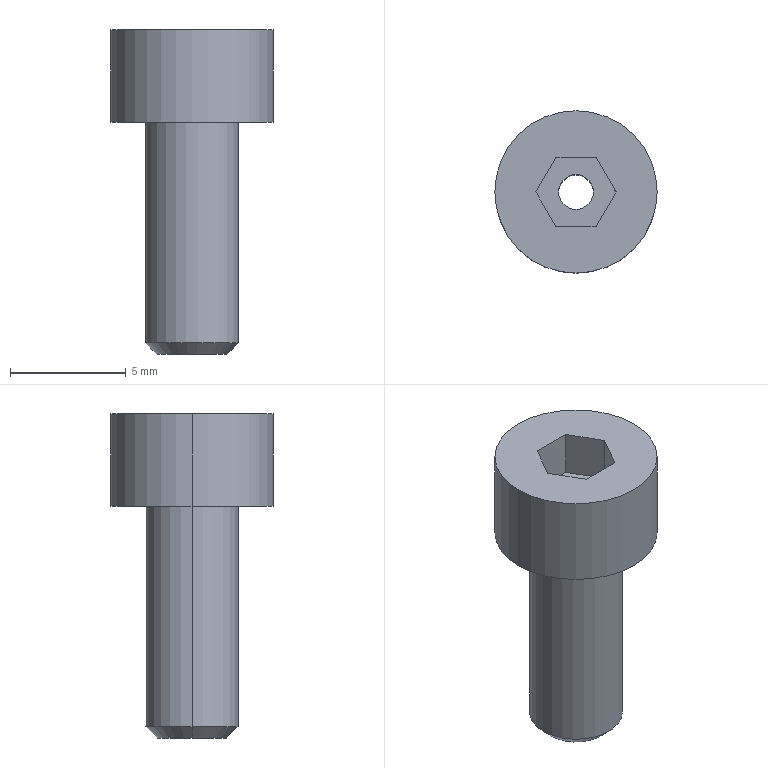Part | SolidWorks | features ICE 3, Chamfer 1, Extrusion 1 | 1 solid | 18 faces | box 7 x 7 x 14 mm | volume 241.368 mm3 | plane 10 | cylinder 6 | cone 2 | commonest cylinder face diameters 1.5 x2 4 x2 7 x2
STEP:
#1=CARTESIAN_POINT('',(-0.75,0.,0.));
#2=VERTEX_POINT('',#1);
#3=CARTESIAN_POINT('',(0.75,0.,0.));
#4=VERTEX_POINT('',#3);
#5=CARTESIAN_POINT('',(0.,0.,0.));
#6=DIRECTION('',(0.,0.,1.));
#7=DIRECTION('',(1.,0.,0.));
#8=AXIS2_PLACEMENT_3D('',#5,#6,#7);
#9=CIRCLE('',#8,0.75);
#10=EDGE_CURVE('',#2,#4,#9,.T.);
#11=ORIENTED_EDGE('',*,*,#10,.F.);
#12=CARTESIAN_POINT('',(-0.75,0.,12.));
#13=VERTEX_POINT('',#12);
#14=CARTESIAN_POINT('',(-0.75,0.,0.));
#15=DIRECTION('',(0.,0.,1.));
#16=VECTOR('',#15,1000.);
#17=LINE('',#14,#16);
#18=EDGE_CURVE('',#2,#13,#17,.T.);
#19=ORIENTED_EDGE('',*,*,#18,.T.);
#20=CARTESIAN_POINT('',(0.75,0.,12.));
#21=VERTEX_POINT('',#20);
#22=CARTESIAN_POINT('',(0.,0.,12.));
#23=DIRECTION('',(0.,0.,1.));
#24=DIRECTION('',(1.,0.,0.));
#25=AXIS2_PLACEMENT_3D('',#22,#23,#24);
#26=CIRCLE('',#25,0.75);
#27=EDGE_CURVE('',#13,#21,#26,.T.);
#28=ORIENTED_EDGE('',*,*,#27,.T.);
#29=CARTESIAN_POINT('',(0.75,0.,0.));
#30=DIRECTION('',(0.,0.,1.));
#31=VECTOR('',#30,1000.);
#32=LINE('',#29,#31);
#33=EDGE_CURVE('',#4,#21,#32,.T.);
#34=ORIENTED_EDGE('',*,*,#33,.F.);
#35=EDGE_LOOP('',(#11,#19,#28,#34));
#36=FACE_OUTER_BOUND('',#35,.T.);
#37=CARTESIAN_POINT('',(0.,0.,0.));
#38=DIRECTION('',(0.,0.,1.));
#39=DIRECTION('',(1.,0.,0.));
#40=AXIS2_PLACEMENT_3D('',#37,#38,#39);
#41=CYLINDRICAL_SURFACE('',#40,0.75);
#42=ADVANCED_FACE('',(#36),#41,.F.);
#43=CARTESIAN_POINT('',(-1.5,0.,0.));
#44=VERTEX_POINT('',#43);
#45=CARTESIAN_POINT('',(1.5,0.,0.));
#46=VERTEX_POINT('',#45);
#47=CARTESIAN_POINT('',(0.,0.,0.));
#48=DIRECTION('',(0.,0.,-1.));
#49=DIRECTION('',(1.,0.,0.));
#50=AXIS2_PLACEMENT_3D('',#47,#48,#49);
#51=CIRCLE('',#50,1.5);
#52=EDGE_CURVE('',#44,#46,#51,.T.);
#53=ORIENTED_EDGE('',*,*,#52,.F.);
#54=CARTESIAN_POINT('',(-2.,0.,0.5));
#55=VERTEX_POINT('',#54);
#56=CARTESIAN_POINT('',(-2.,0.,0.5));
#57=DIRECTION('',(-0.7071,0.,0.7071));
#58=VECTOR('',#57,1000.);
#59=LINE('',#56,#58);
#60=EDGE_CURVE('',#44,#55,#59,.T.);
#61=ORIENTED_EDGE('',*,*,#60,.T.);
#62=CARTESIAN_POINT('',(2.,0.,0.5));
#63=VERTEX_POINT('',#62);
#64=CARTESIAN_POINT('',(0.,0.,0.5));
#65=DIRECTION('',(0.,0.,1.));
#66=DIRECTION('',(1.,0.,0.));
#67=AXIS2_PLACEMENT_3D('',#64,#65,#66);
#68=CIRCLE('',#67,2.);
#69=EDGE_CURVE('',#63,#55,#68,.T.);
#70=ORIENTED_EDGE('',*,*,#69,.F.);
#71=CARTESIAN_POINT('',(2.,0.,0.5));
#72=DIRECTION('',(0.7071,0.,0.7071));
#73=VECTOR('',#72,1000.);
#74=LINE('',#71,#73);
#75=EDGE_CURVE('',#46,#63,#74,.T.);
#76=ORIENTED_EDGE('',*,*,#75,.F.);
#77=EDGE_LOOP('',(#53,#61,#70,#76));
#78=FACE_OUTER_BOUND('',#77,.T.);
#79=CARTESIAN_POINT('',(0.,0.,0.5));
#80=DIRECTION('',(0.,0.,1.));
#81=DIRECTION('',(1.,0.,0.));
#82=AXIS2_PLACEMENT_3D('',#79,#80,#81);
#83=CONICAL_SURFACE('',#82,2.,0.7854);
#84=ADVANCED_FACE('',(#78),#83,.T.);
#85=CARTESIAN_POINT('',(3.5,0.,14.));
#86=VERTEX_POINT('',#85);
#87=CARTESIAN_POINT('',(-3.5,0.,14.));
#88=VERTEX_POINT('',#87);
#89=CARTESIAN_POINT('',(0.,0.,14.));
#90=DIRECTION('',(0.,0.,1.));
#91=DIRECTION('',(1.,0.,0.));
#92=AXIS2_PLACEMENT_3D('',#89,#90,#91);
#93=CIRCLE('',#92,3.5);
#94=EDGE_CURVE('',#86,#88,#93,.T.);
#95=ORIENTED_EDGE('',*,*,#94,.F.);
#96=CARTESIAN_POINT('',(3.5,0.,10.));
#97=VERTEX_POINT('',#96);
#98=CARTESIAN_POINT('',(3.5,0.,14.));
#99=DIRECTION('',(0.,0.,-1.));
#100=VECTOR('',#99,1000.);
#101=LINE('',#98,#100);
#102=EDGE_CURVE('',#86,#97,#101,.T.);
#103=ORIENTED_EDGE('',*,*,#102,.T.);
#104=CARTESIAN_POINT('',(-3.5,0.,10.));
#105=VERTEX_POINT('',#104);
#106=CARTESIAN_POINT('',(0.,0.,10.));
#107=DIRECTION('',(0.,0.,1.));
#108=DIRECTION('',(1.,0.,0.));
#109=AXIS2_PLACEMENT_3D('',#106,#107,#108);
#110=CIRCLE('',#109,3.5);
#111=EDGE_CURVE('',#97,#105,#110,.T.);
#112=ORIENTED_EDGE('',*,*,#111,.T.);
#113=CARTESIAN_POINT('',(-3.5,0.,14.));
#114=DIRECTION('',(0.,0.,-1.));
#115=VECTOR('',#114,1000.);
#116=LINE('',#113,#115);
#117=EDGE_CURVE('',#88,#105,#116,.T.);
#118=ORIENTED_EDGE('',*,*,#117,.F.);
#119=EDGE_LOOP('',(#95,#103,#112,#118));
#120=FACE_OUTER_BOUND('',#119,.T.);
#121=CARTESIAN_POINT('',(0.,0.,14.));
#122=DIRECTION('',(0.,0.,-1.));
#123=DIRECTION('',(-1.,0.,0.));
#124=AXIS2_PLACEMENT_3D('',#121,#122,#123);
#125=CYLINDRICAL_SURFACE('',#124,3.5);
#126=ADVANCED_FACE('',(#120),#125,.T.);
#127=CARTESIAN_POINT('',(2.,0.,10.));
#128=VERTEX_POINT('',#127);
#129=CARTESIAN_POINT('',(-2.,0.,10.));
#130=VERTEX_POINT('',#129);
#131=CARTESIAN_POINT('',(0.,0.,10.));
#132=DIRECTION('',(0.,0.,1.));
#133=DIRECTION('',(1.,0.,0.));
#134=AXIS2_PLACEMENT_3D('',#131,#132,#133);
#135=CIRCLE('',#134,2.);
#136=EDGE_CURVE('',#128,#130,#135,.T.);
#137=ORIENTED_EDGE('',*,*,#136,.F.);
#138=CARTESIAN_POINT('',(2.,0.,10.));
#139=DIRECTION('',(0.,0.,-1.));
#140=VECTOR('',#139,1000.);
#141=LINE('',#138,#140);
#142=EDGE_CURVE('',#128,#63,#141,.T.);
#143=ORIENTED_EDGE('',*,*,#142,.T.);
#144=ORIENTED_EDGE('',*,*,#69,.T.);
#145=CARTESIAN_POINT('',(-2.,0.,10.));
#146=DIRECTION('',(0.,0.,-1.));
#147=VECTOR('',#146,1000.);
#148=LINE('',#145,#147);
#149=EDGE_CURVE('',#130,#55,#148,.T.);
#150=ORIENTED_EDGE('',*,*,#149,.F.);
#151=EDGE_LOOP('',(#137,#143,#144,#150));
#152=FACE_OUTER_BOUND('',#151,.T.);
#153=CARTESIAN_POINT('',(0.,0.,10.));
#154=DIRECTION('',(0.,0.,-1.));
#155=DIRECTION('',(-1.,0.,0.));
#156=AXIS2_PLACEMENT_3D('',#153,#154,#155);
#157=CYLINDRICAL_SURFACE('',#156,2.);
#158=ADVANCED_FACE('',(#152),#157,.T.);
#159=ORIENTED_EDGE('',*,*,#142,.F.);
#160=CARTESIAN_POINT('',(0.,0.,10.));
#161=DIRECTION('',(0.,0.,1.));
#162=DIRECTION('',(1.,0.,0.));
#163=AXIS2_PLACEMENT_3D('',#160,#161,#162);
#164=CIRCLE('',#163,2.);
#165=EDGE_CURVE('',#130,#128,#164,.T.);
#166=ORIENTED_EDGE('',*,*,#165,.F.);
#167=ORIENTED_EDGE('',*,*,#149,.T.);
#168=CARTESIAN_POINT('',(0.,0.,0.5));
#169=DIRECTION('',(0.,0.,1.));
#170=DIRECTION('',(1.,0.,0.));
#171=AXIS2_PLACEMENT_3D('',#168,#169,#170);
#172=CIRCLE('',#171,2.);
#173=EDGE_CURVE('',#55,#63,#172,.T.);
#174=ORIENTED_EDGE('',*,*,#173,.T.);
#175=EDGE_LOOP('',(#159,#166,#167,#174));
#176=FACE_OUTER_BOUND('',#175,.T.);
#177=CARTESIAN_POINT('',(0.,0.,10.));
#178=DIRECTION('',(0.,0.,-1.));
#179=DIRECTION('',(-1.,0.,0.));
#180=AXIS2_PLACEMENT_3D('',#177,#178,#179);
#181=CYLINDRICAL_SURFACE('',#180,2.);
#182=ADVANCED_FACE('',(#176),#181,.T.);
#183=CARTESIAN_POINT('',(0.,0.,0.));
#184=DIRECTION('',(0.,0.,1.));
#185=DIRECTION('',(1.,0.,0.));
#186=AXIS2_PLACEMENT_3D('',#183,#184,#185);
#187=CIRCLE('',#186,0.75);
#188=EDGE_CURVE('',#4,#2,#187,.T.);
#189=ORIENTED_EDGE('',*,*,#188,.T.);
#190=ORIENTED_EDGE('',*,*,#10,.T.);
#191=EDGE_LOOP('',(#189,#190));
#192=FACE_BOUND('',#191,.T.);
#193=CARTESIAN_POINT('',(0.,0.,0.));
#194=DIRECTION('',(0.,0.,-1.));
#195=DIRECTION('',(1.,0.,0.));
#196=AXIS2_PLACEMENT_3D('',#193,#194,#195);
#197=CIRCLE('',#196,1.5);
#198=EDGE_CURVE('',#46,#44,#197,.T.);
#199=ORIENTED_EDGE('',*,*,#198,.T.);
#200=ORIENTED_EDGE('',*,*,#52,.T.);
#201=EDGE_LOOP('',(#199,#200));
#202=FACE_OUTER_BOUND('',#201,.T.);
#203=CARTESIAN_POINT('',(0.,0.,0.));
#204=DIRECTION('',(0.,0.,1.));
#205=DIRECTION('',(1.,0.,0.));
#206=AXIS2_PLACEMENT_3D('',#203,#204,#205);
#207=PLANE('',#206);
#208=ADVANCED_FACE('',(#192,#202),#207,.F.);
#209=ORIENTED_EDGE('',*,*,#102,.F.);
#210=CARTESIAN_POINT('',(0.,0.,14.));
#211=DIRECTION('',(0.,0.,1.));
#212=DIRECTION('',(1.,0.,0.));
#213=AXIS2_PLACEMENT_3D('',#210,#211,#212);
#214=CIRCLE('',#213,3.5);
#215=EDGE_CURVE('',#88,#86,#214,.T.);
#216=ORIENTED_EDGE('',*,*,#215,.F.);
#217=ORIENTED_EDGE('',*,*,#117,.T.);
#218=CARTESIAN_POINT('',(0.,0.,10.));
#219=DIRECTION('',(0.,0.,1.));
#220=DIRECTION('',(1.,0.,0.));
#221=AXIS2_PLACEMENT_3D('',#218,#219,#220);
#222=CIRCLE('',#221,3.5);
#223=EDGE_CURVE('',#105,#97,#222,.T.);
#224=ORIENTED_EDGE('',*,*,#223,.T.);
#225=EDGE_LOOP('',(#209,#216,#217,#224));
#226=FACE_OUTER_BOUND('',#225,.T.);
#227=CARTESIAN_POINT('',(0.,0.,14.));
#228=DIRECTION('',(0.,0.,-1.));
#229=DIRECTION('',(-1.,0.,0.));
#230=AXIS2_PLACEMENT_3D('',#227,#228,#229);
#231=CYLINDRICAL_SURFACE('',#230,3.5);
#232=ADVANCED_FACE('',(#226),#231,.T.);
#233=CARTESIAN_POINT('',(0.8689,1.498,14.));
#234=VERTEX_POINT('',#233);
#235=CARTESIAN_POINT('',(-0.8632,1.502,14.));
#236=VERTEX_POINT('',#235);
#237=CARTESIAN_POINT('',(0.8689,1.498,14.));
#238=DIRECTION('',(-1.,0.001912,0.));
#239=VECTOR('',#238,1000.);
#240=LINE('',#237,#239);
#241=EDGE_CURVE('',#234,#236,#240,.T.);
#242=ORIENTED_EDGE('',*,*,#241,.F.);
#243=CARTESIAN_POINT('',(1.732,-0.003312,14.));
#244=VERTEX_POINT('',#243);
#245=CARTESIAN_POINT('',(1.732,-0.003312,14.));
#246=DIRECTION('',(-0.4983,0.867,0.));
#247=VECTOR('',#246,1000.);
#248=LINE('',#245,#247);
#249=EDGE_CURVE('',#244,#234,#248,.T.);
#250=ORIENTED_EDGE('',*,*,#249,.F.);
#251=CARTESIAN_POINT('',(0.8632,-1.502,14.));
#252=VERTEX_POINT('',#251);
#253=CARTESIAN_POINT('',(0.8632,-1.502,14.));
#254=DIRECTION('',(0.5017,0.8651,0.));
#255=VECTOR('',#254,1000.);
#256=LINE('',#253,#255);
#257=EDGE_CURVE('',#252,#244,#256,.T.);
#258=ORIENTED_EDGE('',*,*,#257,.F.);
#259=CARTESIAN_POINT('',(-0.8689,-1.498,14.));
#260=VERTEX_POINT('',#259);
#261=CARTESIAN_POINT('',(-0.8689,-1.498,14.));
#262=DIRECTION('',(1.,-0.001912,0.));
#263=VECTOR('',#262,1000.);
#264=LINE('',#261,#263);
#265=EDGE_CURVE('',#260,#252,#264,.T.);
#266=ORIENTED_EDGE('',*,*,#265,.F.);
#267=CARTESIAN_POINT('',(-1.732,0.003312,14.));
#268=VERTEX_POINT('',#267);
#269=CARTESIAN_POINT('',(-1.732,0.003312,14.));
#270=DIRECTION('',(0.4983,-0.867,0.));
#271=VECTOR('',#270,1000.);
#272=LINE('',#269,#271);
#273=EDGE_CURVE('',#268,#260,#272,.T.);
#274=ORIENTED_EDGE('',*,*,#273,.F.);
#275=CARTESIAN_POINT('',(-0.8632,1.502,14.));
#276=DIRECTION('',(-0.5017,-0.8651,0.));
#277=VECTOR('',#276,1000.);
#278=LINE('',#275,#277);
#279=EDGE_CURVE('',#236,#268,#278,.T.);
#280=ORIENTED_EDGE('',*,*,#279,.F.);
#281=EDGE_LOOP('',(#242,#250,#258,#266,#274,#280));
#282=FACE_BOUND('',#281,.T.);
#283=ORIENTED_EDGE('',*,*,#215,.T.);
#284=ORIENTED_EDGE('',*,*,#94,.T.);
#285=EDGE_LOOP('',(#283,#284));
#286=FACE_OUTER_BOUND('',#285,.T.);
#287=CARTESIAN_POINT('',(0.,0.,14.));
#288=DIRECTION('',(0.,0.,1.));
#289=DIRECTION('',(1.,0.,0.));
#290=AXIS2_PLACEMENT_3D('',#287,#288,#289);
#291=PLANE('',#290);
#292=ADVANCED_FACE('',(#282,#286),#291,.T.);
#293=ORIENTED_EDGE('',*,*,#165,.T.);
#294=ORIENTED_EDGE('',*,*,#136,.T.);
#295=EDGE_LOOP('',(#293,#294));
#296=FACE_BOUND('',#295,.T.);
#297=ORIENTED_EDGE('',*,*,#223,.F.);
#298=ORIENTED_EDGE('',*,*,#111,.F.);
#299=EDGE_LOOP('',(#297,#298));
#300=FACE_OUTER_BOUND('',#299,.T.);
#301=CARTESIAN_POINT('',(0.,0.,10.));
#302=DIRECTION('',(0.,0.,1.));
#303=DIRECTION('',(1.,0.,0.));
#304=AXIS2_PLACEMENT_3D('',#301,#302,#303);
#305=PLANE('',#304);
#306=ADVANCED_FACE('',(#296,#300),#305,.F.);
#307=ORIENTED_EDGE('',*,*,#241,.T.);
#308=CARTESIAN_POINT('',(-0.8632,1.502,12.));
#309=VERTEX_POINT('',#308);
#310=CARTESIAN_POINT('',(-0.8632,1.502,12.));
#311=DIRECTION('',(0.,0.,1.));
#312=VECTOR('',#311,1000.);
#313=LINE('',#310,#312);
#314=EDGE_CURVE('',#309,#236,#313,.T.);
#315=ORIENTED_EDGE('',*,*,#314,.F.);
#316=CARTESIAN_POINT('',(0.8689,1.498,12.));
#317=VERTEX_POINT('',#316);
#318=CARTESIAN_POINT('',(0.8689,1.498,12.));
#319=DIRECTION('',(-1.,0.001912,0.));
#320=VECTOR('',#319,1000.);
#321=LINE('',#318,#320);
#322=EDGE_CURVE('',#317,#309,#321,.T.);
#323=ORIENTED_EDGE('',*,*,#322,.F.);
#324=CARTESIAN_POINT('',(0.8689,1.498,12.));
#325=DIRECTION('',(0.,0.,1.));
#326=VECTOR('',#325,1000.);
#327=LINE('',#324,#326);
#328=EDGE_CURVE('',#317,#234,#327,.T.);
#329=ORIENTED_EDGE('',*,*,#328,.T.);
#330=EDGE_LOOP('',(#307,#315,#323,#329));
#331=FACE_OUTER_BOUND('',#330,.T.);
#332=CARTESIAN_POINT('',(0.8689,1.498,12.));
#333=DIRECTION('',(0.001912,1.,0.));
#334=DIRECTION('',(-1.,0.001912,0.));
#335=AXIS2_PLACEMENT_3D('',#332,#333,#334);
#336=PLANE('',#335);
#337=ADVANCED_FACE('',(#331),#336,.F.);
#338=ORIENTED_EDGE('',*,*,#249,.T.);
#339=ORIENTED_EDGE('',*,*,#328,.F.);
#340=CARTESIAN_POINT('',(1.732,-0.003312,12.));
#341=VERTEX_POINT('',#340);
#342=CARTESIAN_POINT('',(1.732,-0.003312,12.));
#343=DIRECTION('',(-0.4983,0.867,0.));
#344=VECTOR('',#343,1000.);
#345=LINE('',#342,#344);
#346=EDGE_CURVE('',#341,#317,#345,.T.);
#347=ORIENTED_EDGE('',*,*,#346,.F.);
#348=CARTESIAN_POINT('',(1.732,-0.003312,12.));
#349=DIRECTION('',(0.,0.,1.));
#350=VECTOR('',#349,1000.);
#351=LINE('',#348,#350);
#352=EDGE_CURVE('',#341,#244,#351,.T.);
#353=ORIENTED_EDGE('',*,*,#352,.T.);
#354=EDGE_LOOP('',(#338,#339,#347,#353));
#355=FACE_OUTER_BOUND('',#354,.T.);
#356=CARTESIAN_POINT('',(1.732,-0.003312,12.));
#357=DIRECTION('',(0.867,0.4983,0.));
#358=DIRECTION('',(-0.4983,0.867,0.));
#359=AXIS2_PLACEMENT_3D('',#356,#357,#358);
#360=PLANE('',#359);
#361=ADVANCED_FACE('',(#355),#360,.F.);
#362=ORIENTED_EDGE('',*,*,#257,.T.);
#363=ORIENTED_EDGE('',*,*,#352,.F.);
#364=CARTESIAN_POINT('',(0.8632,-1.502,12.));
#365=VERTEX_POINT('',#364);
#366=CARTESIAN_POINT('',(0.8632,-1.502,12.));
#367=DIRECTION('',(0.5017,0.8651,0.));
#368=VECTOR('',#367,1000.);
#369=LINE('',#366,#368);
#370=EDGE_CURVE('',#365,#341,#369,.T.);
#371=ORIENTED_EDGE('',*,*,#370,.F.);
#372=CARTESIAN_POINT('',(0.8632,-1.502,12.));
#373=DIRECTION('',(0.,0.,1.));
#374=VECTOR('',#373,1000.);
#375=LINE('',#372,#374);
#376=EDGE_CURVE('',#365,#252,#375,.T.);
#377=ORIENTED_EDGE('',*,*,#376,.T.);
#378=EDGE_LOOP('',(#362,#363,#371,#377));
#379=FACE_OUTER_BOUND('',#378,.T.);
#380=CARTESIAN_POINT('',(0.8632,-1.502,12.));
#381=DIRECTION('',(0.8651,-0.5017,0.));
#382=DIRECTION('',(0.5017,0.8651,0.));
#383=AXIS2_PLACEMENT_3D('',#380,#381,#382);
#384=PLANE('',#383);
#385=ADVANCED_FACE('',(#379),#384,.F.);
#386=ORIENTED_EDGE('',*,*,#265,.T.);
#387=ORIENTED_EDGE('',*,*,#376,.F.);
#388=CARTESIAN_POINT('',(-0.8689,-1.498,12.));
#389=VERTEX_POINT('',#388);
#390=CARTESIAN_POINT('',(-0.8689,-1.498,12.));
#391=DIRECTION('',(1.,-0.001912,0.));
#392=VECTOR('',#391,1000.);
#393=LINE('',#390,#392);
#394=EDGE_CURVE('',#389,#365,#393,.T.);
#395=ORIENTED_EDGE('',*,*,#394,.F.);
#396=CARTESIAN_POINT('',(-0.8689,-1.498,12.));
#397=DIRECTION('',(0.,0.,1.));
#398=VECTOR('',#397,1000.);
#399=LINE('',#396,#398);
#400=EDGE_CURVE('',#389,#260,#399,.T.);
#401=ORIENTED_EDGE('',*,*,#400,.T.);
#402=EDGE_LOOP('',(#386,#387,#395,#401));
#403=FACE_OUTER_BOUND('',#402,.T.);
#404=CARTESIAN_POINT('',(-0.8689,-1.498,12.));
#405=DIRECTION('',(-0.001912,-1.,0.));
#406=DIRECTION('',(1.,-0.001912,0.));
#407=AXIS2_PLACEMENT_3D('',#404,#405,#406);
#408=PLANE('',#407);
#409=ADVANCED_FACE('',(#403),#408,.F.);
#410=ORIENTED_EDGE('',*,*,#273,.T.);
#411=ORIENTED_EDGE('',*,*,#400,.F.);
#412=CARTESIAN_POINT('',(-1.732,0.003312,12.));
#413=VERTEX_POINT('',#412);
#414=CARTESIAN_POINT('',(-1.732,0.003312,12.));
#415=DIRECTION('',(0.4983,-0.867,0.));
#416=VECTOR('',#415,1000.);
#417=LINE('',#414,#416);
#418=EDGE_CURVE('',#413,#389,#417,.T.);
#419=ORIENTED_EDGE('',*,*,#418,.F.);
#420=CARTESIAN_POINT('',(-1.732,0.003312,12.));
#421=DIRECTION('',(0.,0.,1.));
#422=VECTOR('',#421,1000.);
#423=LINE('',#420,#422);
#424=EDGE_CURVE('',#413,#268,#423,.T.);
#425=ORIENTED_EDGE('',*,*,#424,.T.);
#426=EDGE_LOOP('',(#410,#411,#419,#425));
#427=FACE_OUTER_BOUND('',#426,.T.);
#428=CARTESIAN_POINT('',(-1.732,0.003312,12.));
#429=DIRECTION('',(-0.867,-0.4983,0.));
#430=DIRECTION('',(0.4983,-0.867,0.));
#431=AXIS2_PLACEMENT_3D('',#428,#429,#430);
#432=PLANE('',#431);
#433=ADVANCED_FACE('',(#427),#432,.F.);
#434=ORIENTED_EDGE('',*,*,#279,.T.);
#435=ORIENTED_EDGE('',*,*,#424,.F.);
#436=CARTESIAN_POINT('',(-0.8632,1.502,12.));
#437=DIRECTION('',(-0.5017,-0.8651,0.));
#438=VECTOR('',#437,1000.);
#439=LINE('',#436,#438);
#440=EDGE_CURVE('',#309,#413,#439,.T.);
#441=ORIENTED_EDGE('',*,*,#440,.F.);
#442=ORIENTED_EDGE('',*,*,#314,.T.);
#443=EDGE_LOOP('',(#434,#435,#441,#442));
#444=FACE_OUTER_BOUND('',#443,.T.);
#445=CARTESIAN_POINT('',(-0.8632,1.502,12.));
#446=DIRECTION('',(-0.8651,0.5017,0.));
#447=DIRECTION('',(-0.5017,-0.8651,0.));
#448=AXIS2_PLACEMENT_3D('',#445,#446,#447);
#449=PLANE('',#448);
#450=ADVANCED_FACE('',(#444),#449,.F.);
#451=CARTESIAN_POINT('',(0.,0.,12.));
#452=DIRECTION('',(0.,0.,1.));
#453=DIRECTION('',(1.,0.,0.));
#454=AXIS2_PLACEMENT_3D('',#451,#452,#453);
#455=CIRCLE('',#454,0.75);
#456=EDGE_CURVE('',#21,#13,#455,.T.);
#457=ORIENTED_EDGE('',*,*,#456,.F.);
#458=ORIENTED_EDGE('',*,*,#27,.F.);
#459=EDGE_LOOP('',(#457,#458));
#460=FACE_BOUND('',#459,.T.);
#461=ORIENTED_EDGE('',*,*,#322,.T.);
#462=ORIENTED_EDGE('',*,*,#440,.T.);
#463=ORIENTED_EDGE('',*,*,#418,.T.);
#464=ORIENTED_EDGE('',*,*,#394,.T.);
#465=ORIENTED_EDGE('',*,*,#370,.T.);
#466=ORIENTED_EDGE('',*,*,#346,.T.);
#467=EDGE_LOOP('',(#461,#462,#463,#464,#465,#466));
#468=FACE_OUTER_BOUND('',#467,.T.);
#469=CARTESIAN_POINT('',(0.,0.,12.));
#470=DIRECTION('',(0.,0.,1.));
#471=DIRECTION('',(1.,0.,0.));
#472=AXIS2_PLACEMENT_3D('',#469,#470,#471);
#473=PLANE('',#472);
#474=ADVANCED_FACE('',(#460,#468),#473,.T.);
#475=ORIENTED_EDGE('',*,*,#60,.F.);
#476=ORIENTED_EDGE('',*,*,#198,.F.);
#477=ORIENTED_EDGE('',*,*,#75,.T.);
#478=ORIENTED_EDGE('',*,*,#173,.F.);
#479=EDGE_LOOP('',(#475,#476,#477,#478));
#480=FACE_OUTER_BOUND('',#479,.T.);
#481=CARTESIAN_POINT('',(0.,0.,0.5));
#482=DIRECTION('',(0.,0.,1.));
#483=DIRECTION('',(1.,0.,0.));
#484=AXIS2_PLACEMENT_3D('',#481,#482,#483);
#485=CONICAL_SURFACE('',#484,2.,0.7854);
#486=ADVANCED_FACE('',(#480),#485,.T.);
#487=ORIENTED_EDGE('',*,*,#18,.F.);
#488=ORIENTED_EDGE('',*,*,#188,.F.);
#489=ORIENTED_EDGE('',*,*,#33,.T.);
#490=ORIENTED_EDGE('',*,*,#456,.T.);
#491=EDGE_LOOP('',(#487,#488,#489,#490));
#492=FACE_OUTER_BOUND('',#491,.T.);
#493=CARTESIAN_POINT('',(0.,0.,0.));
#494=DIRECTION('',(0.,0.,1.));
#495=DIRECTION('',(1.,0.,0.));
#496=AXIS2_PLACEMENT_3D('',#493,#494,#495);
#497=CYLINDRICAL_SURFACE('',#496,0.75);
#498=ADVANCED_FACE('',(#492),#497,.F.);
#499=CLOSED_SHELL('',(#42,#84,#126,#158,#182,#208,#232,#292,#306,#337,#361,#385,#409,#433,#450,#474,#486,#498));
#500=MANIFOLD_SOLID_BREP('',#499);
#501=CARTESIAN_POINT('',(0.,0.,0.));
#502=DIRECTION('',(0.,0.,1.));
#503=DIRECTION('',(1.,0.,0.));
#504=AXIS2_PLACEMENT_3D('',#501,#502,#503);
#505=(LENGTH_UNIT()NAMED_UNIT(*)SI_UNIT(.MILLI.,.METRE.));
#506=UNCERTAINTY_MEASURE_WITH_UNIT(LENGTH_MEASURE(0.00001),#505,'','');
#507=(NAMED_UNIT(*)PLANE_ANGLE_UNIT()SI_UNIT($,.RADIAN.));
#508=(NAMED_UNIT(*)SI_UNIT($,.STERADIAN.)SOLID_ANGLE_UNIT());
#509=(GEOMETRIC_REPRESENTATION_CONTEXT(3)GLOBAL_UNCERTAINTY_ASSIGNED_CONTEXT((#506))GLOBAL_UNIT_ASSIGNED_CONTEXT((#505,#507,#508))REPRESENTATION_CONTEXT('',''));
#510=ADVANCED_BREP_SHAPE_REPRESENTATION('',(#500,#504),#509);